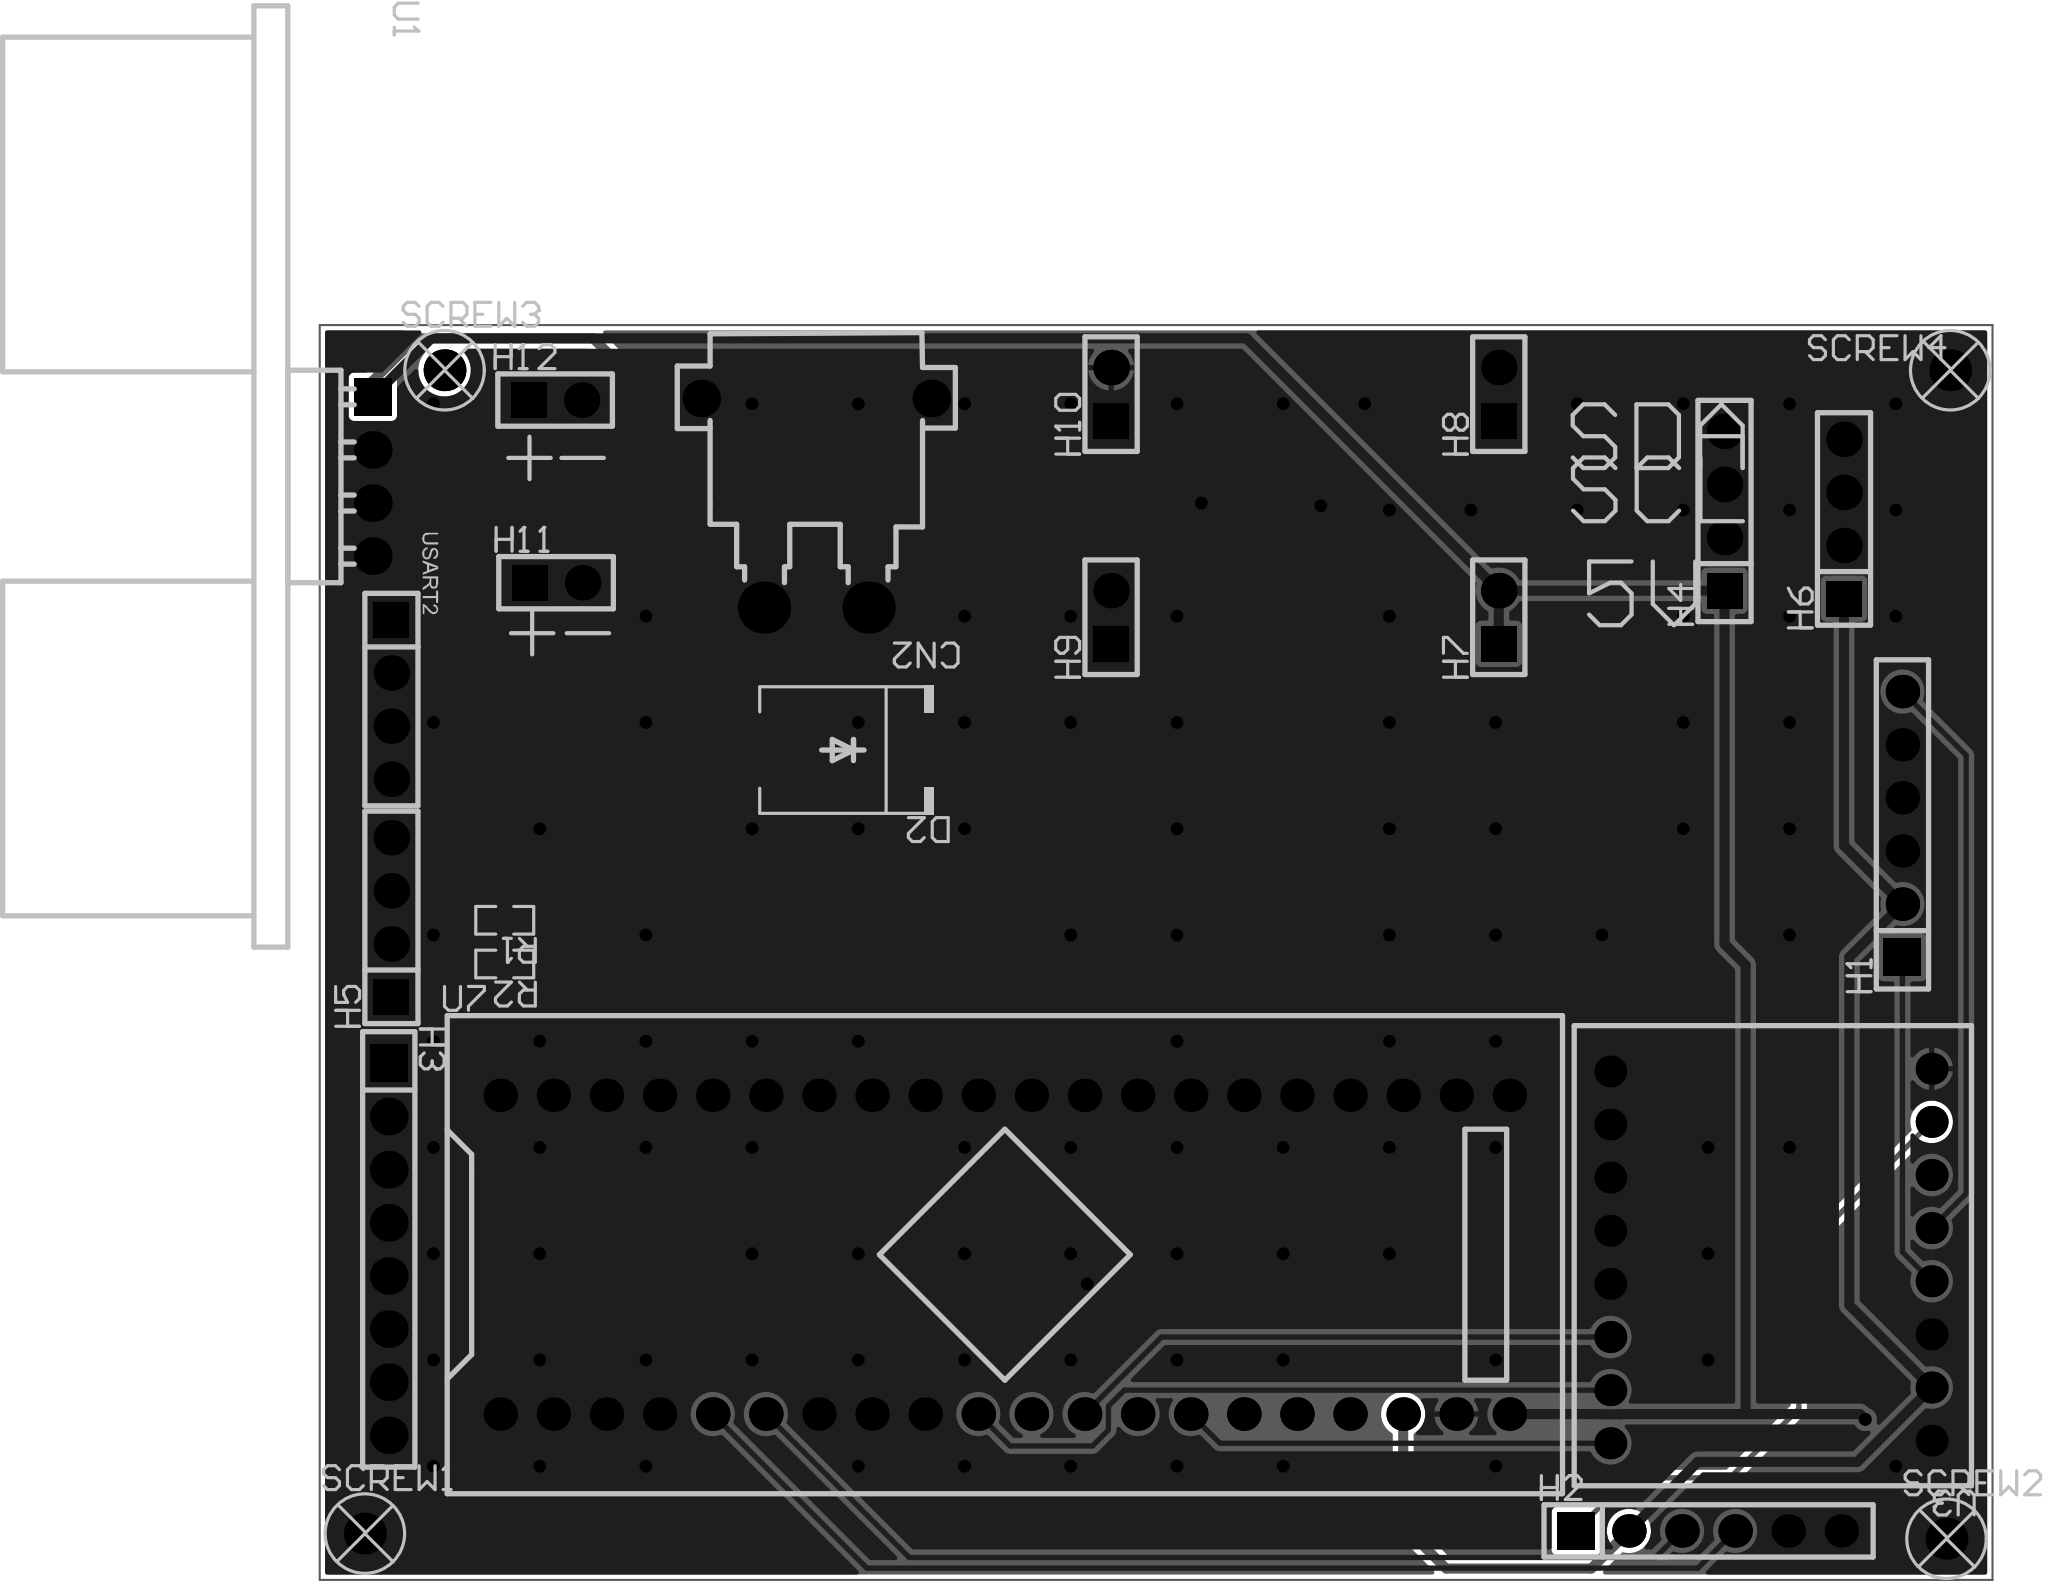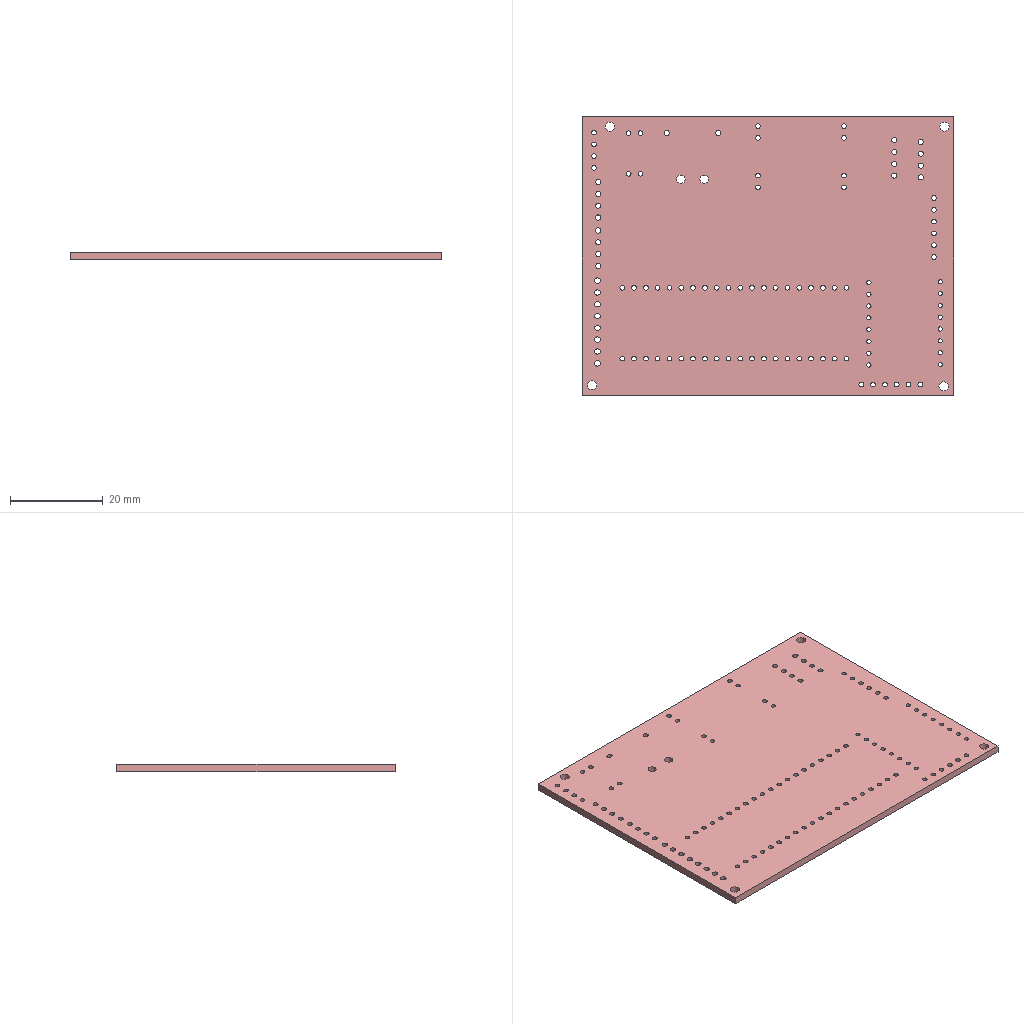Circuit board layout | Altium Designer | box 80 x 60 x 1.6 mm
Layer stack:
# Altium Designer layer stack of  (unit mm; dielectric type: 0 none, 1 core, 2 prepreg, 3 surface material)
index,name,kind,layer,copper_thickness_mm,dielectric_type,dielectric_thickness_mm,dielectric_material,dielectric_constant
0,Top Paste Mask Layer,other,,,,,,
1,Top Silkscreen Layer,other,,,,,,
2,Top Solder Mask Layer,dielectric,,,3,0.01,,3.3
3,Top Layer,copper,Top Layer,0.035,,,,
4,Dielectric1,dielectric,,,3,1.51,FR4,4.5
5,Bottom Layer,copper,Bottom Layer,0.035,,,,
6,Bottom Solder Mask Layer,dielectric,,,3,0.01,,3.3
7,Bottom Silkscreen Layer,other,,,,,,
8,Bottom Paste Mask Layer,other,,,,,,
# drill layer pairs: low layer,high layer
drill_pair,Top Layer,Bottom Layer
Part placement:
Designator,Comment,Layer,Footprint,Center-X(mm),Center-Y(mm),Rotation
CN2,XT30PW-M30.G.Y,TopLayer,CONN-TH_XT30PW-M,132.969,198.374,180
H7,,TopLayer,HDR-TH_2P-P2.54-V-F,165.608,192.913,90
H8,,TopLayer,HDR-TH_2P-P2.54-V-F,165.608,203.581,90
USART2,,TopLayer,HDR-TH_4P-P2.54-V-M,112.649,188.976,270
U7,LCKFB-DKX-STM32F103C8T6,TopLayer,CONN-TH_L53.3-W22.9_STM32F103C8T6-CARD,141.986,162.433,0
H6,,TopLayer,HDR-TH_4P-P2.54-V-M,182.118,197.612,90
H9,,TopLayer,HDR-TH_2P-P2.54-V-F,147.066,192.913,90
H10,,TopLayer,HDR-TH_2P-P2.54-V-F,147.066,203.581,90
H11,,TopLayer,HDR-TH_2P-P2.54-V-F,120.523,194.564,0
H12,,TopLayer,HDR-TH_2P-P2.54-V-F,120.478,203.298,0
H1,,TopLayer,HDR-TH_6P-P2.54-V-F,184.912,183.007,90
H2,,TopLayer,HDR-TH_6P-P2.54-V-F,175.641,149.225,0
U3,,TopLayer,TB6612,178.625,162.369,180
D2,SS34,TopLayer,SMC_L6.9-W5.9-LS7.9-RD,134.239,186.563,180
H3,,TopLayer,HDR-TH_8P-P2.54-V-F-1,112.522,162.687,270
H4,,TopLayer,HDR-TH_4P-P2.54-V-F,176.403,197.993,90
H5,,TopLayer,HDR-TH_4P-P2.54-V-M,112.649,178.562,90
R1,1K,TopLayer,R0603,118.069,178.423,180
R2,2K,TopLayer,R0603,118.069,176.333,180
U1,HC-SR04,TopLayer,TH_HC-SR04V,111.76,199.644,270
SCREW1,,TopLayer,M2螺丝,111.379,149.098,0
SCREW2,,TopLayer,M2螺丝,187.02,148.85,0
SCREW3,,TopLayer,M2螺丝,115.189,204.724,0
SCREW4,,TopLayer,M2螺丝,187.198,204.724,0
Pad and via stacks:
# Altium Designer via and pad stacks of  (unit mm). Each distinct definition once, with the count of objects using it.
# via: kind,start_layer,end_layer,hole_mm,diameter_mm,mode(0 simple;1 top-mid-bottom;2 full stack),diameter_per_layer,count,example_net
# pad: kind,layer,hole_mm,hole_type(0 round;1 square;2 slot),plating,top_size,top_shape(1 round;2 rect;3 octagon;9 rounded rect),mid_size,bottom_size,mode,footprint,size_per_layer,count,example
pad,Multi-Layer,1.8,0,plated,2.5x2.5,1,2.5x2.5,2.5x2.5,0,CONN-TH_XT30PW-M,,2,CN2.1
pad,Multi-Layer,1.1,0,plated,1.8x1.8,1,1.8x1.8,1.8x1.8,0,CONN-TH_XT30PW-M,,2,CN2.3
pad,Multi-Layer,1,0,plated,1.7x1.7,2,1.7x1.7,1.7x1.7,0,HDR-TH_2P-P2.54-V-F,,6,H7.1
pad,Multi-Layer,1,0,plated,1.7x1.7,1,1.7x1.7,1.7x1.7,0,HDR-TH_2P-P2.54-V-F,,6,H7.2
pad,Multi-Layer,1.1,0,plated,1.7x1.7,2,1.7x1.7,1.7x1.7,0,HDR-TH_4P-P2.54-V-M,,3,USART2.1
pad,Multi-Layer,1.1,0,plated,1.7x1.7,1,1.7x1.7,1.7x1.7,0,HDR-TH_4P-P2.54-V-M,,9,USART2.2
pad,Multi-Layer,1,0,plated,1.6x1.6,1,1.6x1.6,1.6x1.6,0,CONN-TH_L53.3-W22.9_STM32F103C8T6-CARD,,40,U7.1
pad,Multi-Layer,1.02,0,plated,1.6x1.6,1,1.6x1.6,1.6x1.6,0,HDR-TH_6P-P2.54-V-F,,10,H1.6
pad,Multi-Layer,1.02,0,plated,1.8x1.8,2,1.8x1.8,1.8x1.8,0,HDR-TH_6P-P2.54-V-F,,2,H1.1
pad,Multi-Layer,0.9144,0,plated,1.524x1.524,1,1.524x1.524,1.524x1.524,0,TB6612,,16,U3.1
pad,Multi-Layer,1.2,0,plated,1.8x1.8,2,1.8x1.8,1.8x1.8,0,HDR-TH_8P-P2.54-V-F-1,,1,H3.1
pad,Multi-Layer,1.2,0,plated,1.8x1.8,1,1.8x1.8,1.8x1.8,0,HDR-TH_8P-P2.54-V-F-1,,7,H3.2
pad,Multi-Layer,1.1,0,plated,1.7x1.7,2,1.7x1.7,1.7x1.7,0,HDR-TH_4P-P2.54-V-F,,1,H4.1
pad,Multi-Layer,1.1,0,plated,1.7x1.7,1,1.7x1.7,1.7x1.7,0,HDR-TH_4P-P2.54-V-F,,3,H4.2
pad,Multi-Layer,1.001,0,plated,1.8x1.8,1,1.8x1.8,1.8x1.8,0,TH_HC-SR04V,,3,U1.4
pad,Multi-Layer,1.001,0,plated,1.8x1.8,2,1.8x1.8,1.8x1.8,0,TH_HC-SR04V,,1,U1.1
pad,Multi-Layer,2,0,plated,2x2,1,2x2,2x2,0,M2\u00C2\u00DD\u00CB\u00BF,,4,SCREW1.1
pad,Top Layer,0,0,plated,2.7x3.3,2,2.7x3.3,2.7x3.3,0,SMC_L6.9-W5.9-LS7.9-RD,,2,D2.2
pad,Top Layer,0,0,plated,0.8065x0.864,2,0.8065x0.864,0.8065x0.864,0,R0603,,4,R1.2
via,Top Layer,Bottom Layer,0.3048,0.61,0,,108,PC15
Copper pours:
name,layer,net,type(0 solid;1 hatched;2 none)
Top Layer-GND,Top Layer,GND,0
Bottom Layer-GND,Bottom Layer,GND,0
Design rules, without the lines most boards share:
# Altium Designer design rules of  (exported by Altium Designer, unit mm)
# columns: name | kind | enabled | priority | scope1 | scope2 | descriptor | typed fields (field=value)
solderMaskExpansion | 13 | enabled | 2 | All | All | Solder Mask Expansion (Expansion =2.008mil) (All) | expansion=0.051